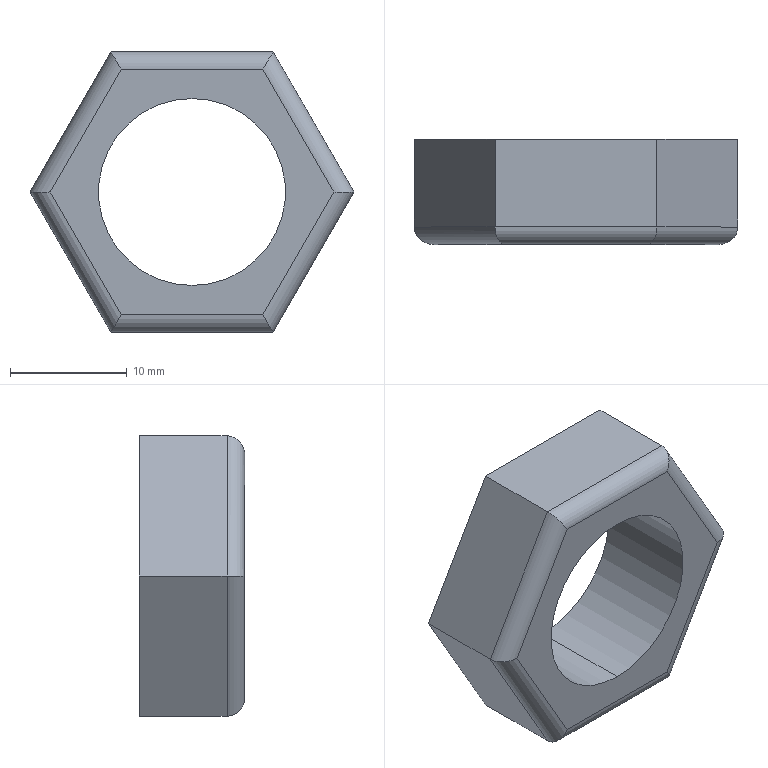Part | SolidWorks | features Extrusion 1, Fillet 1 | 1 solid | 16 faces | box 27.713 x 9 x 24 mm | volume 2641 mm3 | cylinder 8 | plane 8 | commonest cylinder face diameters 3 x6 16 x2
STEP:
#1=CARTESIAN_POINT('',(0.,9.,-8.));
#2=VERTEX_POINT('',#1);
#3=CARTESIAN_POINT('',(0.,9.,8.));
#4=VERTEX_POINT('',#3);
#5=CARTESIAN_POINT('',(0.,9.,0.));
#6=DIRECTION('',(0.,1.,0.));
#7=DIRECTION('',(0.,0.,1.));
#8=AXIS2_PLACEMENT_3D('',#5,#6,#7);
#9=CIRCLE('',#8,8.);
#10=EDGE_CURVE('',#2,#4,#9,.T.);
#11=ORIENTED_EDGE('',*,*,#10,.T.);
#12=CARTESIAN_POINT('',(0.,0.,8.));
#13=VERTEX_POINT('',#12);
#14=CARTESIAN_POINT('',(0.,9.,8.));
#15=DIRECTION('',(0.,-1.,0.));
#16=VECTOR('',#15,1000.);
#17=LINE('',#14,#16);
#18=EDGE_CURVE('',#4,#13,#17,.T.);
#19=ORIENTED_EDGE('',*,*,#18,.T.);
#20=CARTESIAN_POINT('',(0.,0.,-8.));
#21=VERTEX_POINT('',#20);
#22=CARTESIAN_POINT('',(0.,0.,0.));
#23=DIRECTION('',(0.,1.,0.));
#24=DIRECTION('',(0.,0.,1.));
#25=AXIS2_PLACEMENT_3D('',#22,#23,#24);
#26=CIRCLE('',#25,8.);
#27=EDGE_CURVE('',#21,#13,#26,.T.);
#28=ORIENTED_EDGE('',*,*,#27,.F.);
#29=CARTESIAN_POINT('',(0.,9.,-8.));
#30=DIRECTION('',(0.,-1.,0.));
#31=VECTOR('',#30,1000.);
#32=LINE('',#29,#31);
#33=EDGE_CURVE('',#2,#21,#32,.T.);
#34=ORIENTED_EDGE('',*,*,#33,.F.);
#35=EDGE_LOOP('',(#11,#19,#28,#34));
#36=FACE_OUTER_BOUND('',#35,.T.);
#37=CARTESIAN_POINT('',(0.,9.,0.));
#38=DIRECTION('',(0.,-1.,0.));
#39=DIRECTION('',(0.,0.,-1.));
#40=AXIS2_PLACEMENT_3D('',#37,#38,#39);
#41=CYLINDRICAL_SURFACE('',#40,8.);
#42=ADVANCED_FACE('',(#36),#41,.F.);
#43=CARTESIAN_POINT('',(6.928,9.,12.));
#44=VERTEX_POINT('',#43);
#45=CARTESIAN_POINT('',(13.856,9.,0.));
#46=VERTEX_POINT('',#45);
#47=CARTESIAN_POINT('',(6.928,9.,12.));
#48=DIRECTION('',(0.5,0.,-0.866));
#49=VECTOR('',#48,1000.);
#50=LINE('',#47,#49);
#51=EDGE_CURVE('',#44,#46,#50,.T.);
#52=ORIENTED_EDGE('',*,*,#51,.T.);
#53=CARTESIAN_POINT('',(6.928,9.,-12.));
#54=VERTEX_POINT('',#53);
#55=CARTESIAN_POINT('',(13.856,9.,0.));
#56=DIRECTION('',(-0.5,0.,-0.866));
#57=VECTOR('',#56,1000.);
#58=LINE('',#55,#57);
#59=EDGE_CURVE('',#46,#54,#58,.T.);
#60=ORIENTED_EDGE('',*,*,#59,.T.);
#61=CARTESIAN_POINT('',(-6.928,9.,-12.));
#62=VERTEX_POINT('',#61);
#63=CARTESIAN_POINT('',(6.928,9.,-12.));
#64=DIRECTION('',(-1.,0.,0.));
#65=VECTOR('',#64,1000.);
#66=LINE('',#63,#65);
#67=EDGE_CURVE('',#54,#62,#66,.T.);
#68=ORIENTED_EDGE('',*,*,#67,.T.);
#69=CARTESIAN_POINT('',(-13.856,9.,0.));
#70=VERTEX_POINT('',#69);
#71=CARTESIAN_POINT('',(-6.928,9.,-12.));
#72=DIRECTION('',(-0.5,0.,0.866));
#73=VECTOR('',#72,1000.);
#74=LINE('',#71,#73);
#75=EDGE_CURVE('',#62,#70,#74,.T.);
#76=ORIENTED_EDGE('',*,*,#75,.T.);
#77=CARTESIAN_POINT('',(-6.928,9.,12.));
#78=VERTEX_POINT('',#77);
#79=CARTESIAN_POINT('',(-13.856,9.,0.));
#80=DIRECTION('',(0.5,0.,0.866));
#81=VECTOR('',#80,1000.);
#82=LINE('',#79,#81);
#83=EDGE_CURVE('',#70,#78,#82,.T.);
#84=ORIENTED_EDGE('',*,*,#83,.T.);
#85=CARTESIAN_POINT('',(-6.928,9.,12.));
#86=DIRECTION('',(1.,0.,0.));
#87=VECTOR('',#86,1000.);
#88=LINE('',#85,#87);
#89=EDGE_CURVE('',#78,#44,#88,.T.);
#90=ORIENTED_EDGE('',*,*,#89,.T.);
#91=EDGE_LOOP('',(#52,#60,#68,#76,#84,#90));
#92=FACE_OUTER_BOUND('',#91,.T.);
#93=ORIENTED_EDGE('',*,*,#10,.F.);
#94=CARTESIAN_POINT('',(0.,9.,0.));
#95=DIRECTION('',(0.,1.,0.));
#96=DIRECTION('',(0.,0.,1.));
#97=AXIS2_PLACEMENT_3D('',#94,#95,#96);
#98=CIRCLE('',#97,8.);
#99=EDGE_CURVE('',#4,#2,#98,.T.);
#100=ORIENTED_EDGE('',*,*,#99,.F.);
#101=EDGE_LOOP('',(#93,#100));
#102=FACE_BOUND('',#101,.T.);
#103=CARTESIAN_POINT('',(13.856,9.,0.));
#104=DIRECTION('',(0.,1.,0.));
#105=DIRECTION('',(0.,0.,1.));
#106=AXIS2_PLACEMENT_3D('',#103,#104,#105);
#107=PLANE('',#106);
#108=ADVANCED_FACE('',(#92,#102),#107,.T.);
#109=CARTESIAN_POINT('',(-6.062,0.,-10.5));
#110=VERTEX_POINT('',#109);
#111=CARTESIAN_POINT('',(6.062,0.,-10.5));
#112=VERTEX_POINT('',#111);
#113=CARTESIAN_POINT('',(13.856,0.,-10.5));
#114=DIRECTION('',(1.,0.,0.));
#115=VECTOR('',#114,1000.);
#116=LINE('',#113,#115);
#117=EDGE_CURVE('',#110,#112,#116,.T.);
#118=ORIENTED_EDGE('',*,*,#117,.T.);
#119=CARTESIAN_POINT('',(12.124,0.,0.));
#120=VERTEX_POINT('',#119);
#121=CARTESIAN_POINT('',(12.557,0.,0.75));
#122=DIRECTION('',(0.5,0.,0.866));
#123=VECTOR('',#122,1000.);
#124=LINE('',#121,#123);
#125=EDGE_CURVE('',#112,#120,#124,.T.);
#126=ORIENTED_EDGE('',*,*,#125,.T.);
#127=CARTESIAN_POINT('',(6.062,0.,10.5));
#128=VERTEX_POINT('',#127);
#129=CARTESIAN_POINT('',(12.557,0.,-0.75));
#130=DIRECTION('',(-0.5,0.,0.866));
#131=VECTOR('',#130,1000.);
#132=LINE('',#129,#131);
#133=EDGE_CURVE('',#120,#128,#132,.T.);
#134=ORIENTED_EDGE('',*,*,#133,.T.);
#135=CARTESIAN_POINT('',(-6.062,0.,10.5));
#136=VERTEX_POINT('',#135);
#137=CARTESIAN_POINT('',(13.856,0.,10.5));
#138=DIRECTION('',(-1.,0.,0.));
#139=VECTOR('',#138,1000.);
#140=LINE('',#137,#139);
#141=EDGE_CURVE('',#128,#136,#140,.T.);
#142=ORIENTED_EDGE('',*,*,#141,.T.);
#143=CARTESIAN_POINT('',(-12.124,0.,0.));
#144=VERTEX_POINT('',#143);
#145=CARTESIAN_POINT('',(-5.629,0.,11.25));
#146=DIRECTION('',(-0.5,0.,-0.866));
#147=VECTOR('',#146,1000.);
#148=LINE('',#145,#147);
#149=EDGE_CURVE('',#136,#144,#148,.T.);
#150=ORIENTED_EDGE('',*,*,#149,.T.);
#151=CARTESIAN_POINT('',(-5.629,0.,-11.25));
#152=DIRECTION('',(0.5,0.,-0.866));
#153=VECTOR('',#152,1000.);
#154=LINE('',#151,#153);
#155=EDGE_CURVE('',#144,#110,#154,.T.);
#156=ORIENTED_EDGE('',*,*,#155,.T.);
#157=EDGE_LOOP('',(#118,#126,#134,#142,#150,#156));
#158=FACE_OUTER_BOUND('',#157,.T.);
#159=ORIENTED_EDGE('',*,*,#27,.T.);
#160=CARTESIAN_POINT('',(0.,0.,0.));
#161=DIRECTION('',(0.,1.,0.));
#162=DIRECTION('',(0.,0.,1.));
#163=AXIS2_PLACEMENT_3D('',#160,#161,#162);
#164=CIRCLE('',#163,8.);
#165=EDGE_CURVE('',#13,#21,#164,.T.);
#166=ORIENTED_EDGE('',*,*,#165,.T.);
#167=EDGE_LOOP('',(#159,#166));
#168=FACE_BOUND('',#167,.T.);
#169=CARTESIAN_POINT('',(13.856,0.,0.));
#170=DIRECTION('',(0.,1.,0.));
#171=DIRECTION('',(0.,0.,1.));
#172=AXIS2_PLACEMENT_3D('',#169,#170,#171);
#173=PLANE('',#172);
#174=ADVANCED_FACE('',(#158,#168),#173,.F.);
#175=CARTESIAN_POINT('',(6.928,1.5,12.));
#176=VERTEX_POINT('',#175);
#177=CARTESIAN_POINT('',(6.928,9.,12.));
#178=DIRECTION('',(0.,-1.,0.));
#179=VECTOR('',#178,1000.);
#180=LINE('',#177,#179);
#181=EDGE_CURVE('',#44,#176,#180,.T.);
#182=ORIENTED_EDGE('',*,*,#181,.T.);
#183=CARTESIAN_POINT('',(13.856,1.5,0.));
#184=VERTEX_POINT('',#183);
#185=CARTESIAN_POINT('',(6.928,1.5,12.));
#186=DIRECTION('',(0.5,0.,-0.866));
#187=VECTOR('',#186,1000.);
#188=LINE('',#185,#187);
#189=EDGE_CURVE('',#176,#184,#188,.T.);
#190=ORIENTED_EDGE('',*,*,#189,.T.);
#191=CARTESIAN_POINT('',(13.856,9.,0.));
#192=DIRECTION('',(0.,-1.,0.));
#193=VECTOR('',#192,1000.);
#194=LINE('',#191,#193);
#195=EDGE_CURVE('',#46,#184,#194,.T.);
#196=ORIENTED_EDGE('',*,*,#195,.F.);
#197=ORIENTED_EDGE('',*,*,#51,.F.);
#198=EDGE_LOOP('',(#182,#190,#196,#197));
#199=FACE_OUTER_BOUND('',#198,.T.);
#200=CARTESIAN_POINT('',(6.928,9.,12.));
#201=DIRECTION('',(-0.866,0.,-0.5));
#202=DIRECTION('',(-0.5,0.,0.866));
#203=AXIS2_PLACEMENT_3D('',#200,#201,#202);
#204=PLANE('',#203);
#205=ADVANCED_FACE('',(#199),#204,.F.);
#206=ORIENTED_EDGE('',*,*,#195,.T.);
#207=CARTESIAN_POINT('',(6.928,1.5,-12.));
#208=VERTEX_POINT('',#207);
#209=CARTESIAN_POINT('',(13.856,1.5,0.));
#210=DIRECTION('',(-0.5,0.,-0.866));
#211=VECTOR('',#210,1000.);
#212=LINE('',#209,#211);
#213=EDGE_CURVE('',#184,#208,#212,.T.);
#214=ORIENTED_EDGE('',*,*,#213,.T.);
#215=CARTESIAN_POINT('',(6.928,9.,-12.));
#216=DIRECTION('',(0.,-1.,0.));
#217=VECTOR('',#216,1000.);
#218=LINE('',#215,#217);
#219=EDGE_CURVE('',#54,#208,#218,.T.);
#220=ORIENTED_EDGE('',*,*,#219,.F.);
#221=ORIENTED_EDGE('',*,*,#59,.F.);
#222=EDGE_LOOP('',(#206,#214,#220,#221));
#223=FACE_OUTER_BOUND('',#222,.T.);
#224=CARTESIAN_POINT('',(13.856,9.,0.));
#225=DIRECTION('',(-0.866,0.,0.5));
#226=DIRECTION('',(0.5,0.,0.866));
#227=AXIS2_PLACEMENT_3D('',#224,#225,#226);
#228=PLANE('',#227);
#229=ADVANCED_FACE('',(#223),#228,.F.);
#230=ORIENTED_EDGE('',*,*,#219,.T.);
#231=CARTESIAN_POINT('',(-6.928,1.5,-12.));
#232=VERTEX_POINT('',#231);
#233=CARTESIAN_POINT('',(6.928,1.5,-12.));
#234=DIRECTION('',(-1.,0.,0.));
#235=VECTOR('',#234,1000.);
#236=LINE('',#233,#235);
#237=EDGE_CURVE('',#208,#232,#236,.T.);
#238=ORIENTED_EDGE('',*,*,#237,.T.);
#239=CARTESIAN_POINT('',(-6.928,9.,-12.));
#240=DIRECTION('',(0.,-1.,0.));
#241=VECTOR('',#240,1000.);
#242=LINE('',#239,#241);
#243=EDGE_CURVE('',#62,#232,#242,.T.);
#244=ORIENTED_EDGE('',*,*,#243,.F.);
#245=ORIENTED_EDGE('',*,*,#67,.F.);
#246=EDGE_LOOP('',(#230,#238,#244,#245));
#247=FACE_OUTER_BOUND('',#246,.T.);
#248=CARTESIAN_POINT('',(6.928,9.,-12.));
#249=DIRECTION('',(0.,0.,1.));
#250=DIRECTION('',(1.,0.,0.));
#251=AXIS2_PLACEMENT_3D('',#248,#249,#250);
#252=PLANE('',#251);
#253=ADVANCED_FACE('',(#247),#252,.F.);
#254=ORIENTED_EDGE('',*,*,#243,.T.);
#255=CARTESIAN_POINT('',(-13.856,1.5,0.));
#256=VERTEX_POINT('',#255);
#257=CARTESIAN_POINT('',(-6.928,1.5,-12.));
#258=DIRECTION('',(-0.5,0.,0.866));
#259=VECTOR('',#258,1000.);
#260=LINE('',#257,#259);
#261=EDGE_CURVE('',#232,#256,#260,.T.);
#262=ORIENTED_EDGE('',*,*,#261,.T.);
#263=CARTESIAN_POINT('',(-13.856,9.,0.));
#264=DIRECTION('',(0.,-1.,0.));
#265=VECTOR('',#264,1000.);
#266=LINE('',#263,#265);
#267=EDGE_CURVE('',#70,#256,#266,.T.);
#268=ORIENTED_EDGE('',*,*,#267,.F.);
#269=ORIENTED_EDGE('',*,*,#75,.F.);
#270=EDGE_LOOP('',(#254,#262,#268,#269));
#271=FACE_OUTER_BOUND('',#270,.T.);
#272=CARTESIAN_POINT('',(-6.928,9.,-12.));
#273=DIRECTION('',(0.866,0.,0.5));
#274=DIRECTION('',(0.5,0.,-0.866));
#275=AXIS2_PLACEMENT_3D('',#272,#273,#274);
#276=PLANE('',#275);
#277=ADVANCED_FACE('',(#271),#276,.F.);
#278=ORIENTED_EDGE('',*,*,#267,.T.);
#279=CARTESIAN_POINT('',(-6.928,1.5,12.));
#280=VERTEX_POINT('',#279);
#281=CARTESIAN_POINT('',(-13.856,1.5,0.));
#282=DIRECTION('',(0.5,0.,0.866));
#283=VECTOR('',#282,1000.);
#284=LINE('',#281,#283);
#285=EDGE_CURVE('',#256,#280,#284,.T.);
#286=ORIENTED_EDGE('',*,*,#285,.T.);
#287=CARTESIAN_POINT('',(-6.928,9.,12.));
#288=DIRECTION('',(0.,-1.,0.));
#289=VECTOR('',#288,1000.);
#290=LINE('',#287,#289);
#291=EDGE_CURVE('',#78,#280,#290,.T.);
#292=ORIENTED_EDGE('',*,*,#291,.F.);
#293=ORIENTED_EDGE('',*,*,#83,.F.);
#294=EDGE_LOOP('',(#278,#286,#292,#293));
#295=FACE_OUTER_BOUND('',#294,.T.);
#296=CARTESIAN_POINT('',(-13.856,9.,0.));
#297=DIRECTION('',(0.866,0.,-0.5));
#298=DIRECTION('',(-0.5,0.,-0.866));
#299=AXIS2_PLACEMENT_3D('',#296,#297,#298);
#300=PLANE('',#299);
#301=ADVANCED_FACE('',(#295),#300,.F.);
#302=ORIENTED_EDGE('',*,*,#291,.T.);
#303=CARTESIAN_POINT('',(-6.928,1.5,12.));
#304=DIRECTION('',(1.,0.,0.));
#305=VECTOR('',#304,1000.);
#306=LINE('',#303,#305);
#307=EDGE_CURVE('',#280,#176,#306,.T.);
#308=ORIENTED_EDGE('',*,*,#307,.T.);
#309=ORIENTED_EDGE('',*,*,#181,.F.);
#310=ORIENTED_EDGE('',*,*,#89,.F.);
#311=EDGE_LOOP('',(#302,#308,#309,#310));
#312=FACE_OUTER_BOUND('',#311,.T.);
#313=CARTESIAN_POINT('',(-6.928,9.,12.));
#314=DIRECTION('',(0.,0.,-1.));
#315=DIRECTION('',(-1.,0.,0.));
#316=AXIS2_PLACEMENT_3D('',#313,#314,#315);
#317=PLANE('',#316);
#318=ADVANCED_FACE('',(#312),#317,.F.);
#319=ORIENTED_EDGE('',*,*,#18,.F.);
#320=ORIENTED_EDGE('',*,*,#99,.T.);
#321=ORIENTED_EDGE('',*,*,#33,.T.);
#322=ORIENTED_EDGE('',*,*,#165,.F.);
#323=EDGE_LOOP('',(#319,#320,#321,#322));
#324=FACE_OUTER_BOUND('',#323,.T.);
#325=CARTESIAN_POINT('',(0.,9.,0.));
#326=DIRECTION('',(0.,-1.,0.));
#327=DIRECTION('',(0.,0.,-1.));
#328=AXIS2_PLACEMENT_3D('',#325,#326,#327);
#329=CYLINDRICAL_SURFACE('',#328,8.);
#330=ADVANCED_FACE('',(#324),#329,.F.);
#331=CARTESIAN_POINT('',(-12.124,0.,0.));
#332=CARTESIAN_POINT('',(-13.139,0.,0.));
#333=CARTESIAN_POINT('',(-13.856,0.6213,0.));
#334=CARTESIAN_POINT('',(-13.856,1.5,0.));
#335=(BOUNDED_CURVE()B_SPLINE_CURVE(3,(#331,#332,#333,#334),.UNSPECIFIED.,.F.,.T.)B_SPLINE_CURVE_WITH_KNOTS((4,4),(4.712,6.283),.UNSPECIFIED.)CURVE()GEOMETRIC_REPRESENTATION_ITEM()RATIONAL_B_SPLINE_CURVE((1.,0.8047,0.8047,1.))REPRESENTATION_ITEM(''));
#336=EDGE_CURVE('',#144,#256,#335,.T.);
#337=ORIENTED_EDGE('',*,*,#336,.F.);
#338=ORIENTED_EDGE('',*,*,#149,.F.);
#339=CARTESIAN_POINT('',(-6.928,1.5,12.));
#340=CARTESIAN_POINT('',(-6.928,0.6213,12.));
#341=CARTESIAN_POINT('',(-6.569,0.,11.379));
#342=CARTESIAN_POINT('',(-6.062,0.,10.5));
#343=(BOUNDED_CURVE()B_SPLINE_CURVE(3,(#339,#340,#341,#342),.UNSPECIFIED.,.F.,.F.)B_SPLINE_CURVE_WITH_KNOTS((4,4),(0.,1.571),.UNSPECIFIED.)CURVE()GEOMETRIC_REPRESENTATION_ITEM()RATIONAL_B_SPLINE_CURVE((1.,0.8047,0.8047,1.))REPRESENTATION_ITEM(''));
#344=EDGE_CURVE('',#280,#136,#343,.T.);
#345=ORIENTED_EDGE('',*,*,#344,.F.);
#346=ORIENTED_EDGE('',*,*,#285,.F.);
#347=EDGE_LOOP('',(#337,#338,#345,#346));
#348=FACE_OUTER_BOUND('',#347,.T.);
#349=CARTESIAN_POINT('',(-12.557,1.5,-0.75));
#350=DIRECTION('',(0.5,0.,0.866));
#351=DIRECTION('',(0.866,0.,-0.5));
#352=AXIS2_PLACEMENT_3D('',#349,#350,#351);
#353=CYLINDRICAL_SURFACE('',#352,1.5);
#354=ADVANCED_FACE('',(#348),#353,.T.);
#355=ORIENTED_EDGE('',*,*,#344,.T.);
#356=ORIENTED_EDGE('',*,*,#141,.F.);
#357=CARTESIAN_POINT('',(6.928,1.5,12.));
#358=CARTESIAN_POINT('',(6.928,0.6213,12.));
#359=CARTESIAN_POINT('',(6.569,0.,11.379));
#360=CARTESIAN_POINT('',(6.062,0.,10.5));
#361=(BOUNDED_CURVE()B_SPLINE_CURVE(3,(#357,#358,#359,#360),.UNSPECIFIED.,.F.,.F.)B_SPLINE_CURVE_WITH_KNOTS((4,4),(0.,1.571),.UNSPECIFIED.)CURVE()GEOMETRIC_REPRESENTATION_ITEM()RATIONAL_B_SPLINE_CURVE((1.,0.8047,0.8047,1.))REPRESENTATION_ITEM(''));
#362=EDGE_CURVE('',#176,#128,#361,.T.);
#363=ORIENTED_EDGE('',*,*,#362,.F.);
#364=ORIENTED_EDGE('',*,*,#307,.F.);
#365=EDGE_LOOP('',(#355,#356,#363,#364));
#366=FACE_OUTER_BOUND('',#365,.T.);
#367=CARTESIAN_POINT('',(-6.928,1.5,10.5));
#368=DIRECTION('',(1.,0.,0.));
#369=DIRECTION('',(0.,0.,-1.));
#370=AXIS2_PLACEMENT_3D('',#367,#368,#369);
#371=CYLINDRICAL_SURFACE('',#370,1.5);
#372=ADVANCED_FACE('',(#366),#371,.T.);
#373=ORIENTED_EDGE('',*,*,#336,.T.);
#374=ORIENTED_EDGE('',*,*,#261,.F.);
#375=CARTESIAN_POINT('',(-6.062,0.,-10.5));
#376=CARTESIAN_POINT('',(-6.569,0.,-11.379));
#377=CARTESIAN_POINT('',(-6.928,0.6213,-12.));
#378=CARTESIAN_POINT('',(-6.928,1.5,-12.));
#379=(BOUNDED_CURVE()B_SPLINE_CURVE(3,(#375,#376,#377,#378),.UNSPECIFIED.,.F.,.F.)B_SPLINE_CURVE_WITH_KNOTS((4,4),(4.712,6.283),.UNSPECIFIED.)CURVE()GEOMETRIC_REPRESENTATION_ITEM()RATIONAL_B_SPLINE_CURVE((1.,0.8047,0.8047,1.))REPRESENTATION_ITEM(''));
#380=EDGE_CURVE('',#110,#232,#379,.T.);
#381=ORIENTED_EDGE('',*,*,#380,.F.);
#382=ORIENTED_EDGE('',*,*,#155,.F.);
#383=EDGE_LOOP('',(#373,#374,#381,#382));
#384=FACE_OUTER_BOUND('',#383,.T.);
#385=CARTESIAN_POINT('',(-5.629,1.5,-11.25));
#386=DIRECTION('',(-0.5,0.,0.866));
#387=DIRECTION('',(0.866,0.,0.5));
#388=AXIS2_PLACEMENT_3D('',#385,#386,#387);
#389=CYLINDRICAL_SURFACE('',#388,1.5);
#390=ADVANCED_FACE('',(#384),#389,.T.);
#391=ORIENTED_EDGE('',*,*,#362,.T.);
#392=ORIENTED_EDGE('',*,*,#133,.F.);
#393=CARTESIAN_POINT('',(13.856,1.5,0.));
#394=CARTESIAN_POINT('',(13.856,0.6213,0.));
#395=CARTESIAN_POINT('',(13.139,0.,0.));
#396=CARTESIAN_POINT('',(12.124,0.,0.));
#397=(BOUNDED_CURVE()B_SPLINE_CURVE(3,(#393,#394,#395,#396),.UNSPECIFIED.,.F.,.T.)B_SPLINE_CURVE_WITH_KNOTS((4,4),(0.,1.571),.UNSPECIFIED.)CURVE()GEOMETRIC_REPRESENTATION_ITEM()RATIONAL_B_SPLINE_CURVE((1.,0.8047,0.8047,1.))REPRESENTATION_ITEM(''));
#398=EDGE_CURVE('',#184,#120,#397,.T.);
#399=ORIENTED_EDGE('',*,*,#398,.F.);
#400=ORIENTED_EDGE('',*,*,#189,.F.);
#401=EDGE_LOOP('',(#391,#392,#399,#400));
#402=FACE_OUTER_BOUND('',#401,.T.);
#403=CARTESIAN_POINT('',(5.629,1.5,11.25));
#404=DIRECTION('',(0.5,0.,-0.866));
#405=DIRECTION('',(-0.866,0.,-0.5));
#406=AXIS2_PLACEMENT_3D('',#403,#404,#405);
#407=CYLINDRICAL_SURFACE('',#406,1.5);
#408=ADVANCED_FACE('',(#402),#407,.T.);
#409=ORIENTED_EDGE('',*,*,#380,.T.);
#410=ORIENTED_EDGE('',*,*,#237,.F.);
#411=CARTESIAN_POINT('',(6.062,0.,-10.5));
#412=CARTESIAN_POINT('',(6.569,0.,-11.379));
#413=CARTESIAN_POINT('',(6.928,0.6213,-12.));
#414=CARTESIAN_POINT('',(6.928,1.5,-12.));
#415=(BOUNDED_CURVE()B_SPLINE_CURVE(3,(#411,#412,#413,#414),.UNSPECIFIED.,.F.,.F.)B_SPLINE_CURVE_WITH_KNOTS((4,4),(1.571,3.142),.UNSPECIFIED.)CURVE()GEOMETRIC_REPRESENTATION_ITEM()RATIONAL_B_SPLINE_CURVE((1.,0.8047,0.8047,1.))REPRESENTATION_ITEM(''));
#416=EDGE_CURVE('',#112,#208,#415,.T.);
#417=ORIENTED_EDGE('',*,*,#416,.F.);
#418=ORIENTED_EDGE('',*,*,#117,.F.);
#419=EDGE_LOOP('',(#409,#410,#417,#418));
#420=FACE_OUTER_BOUND('',#419,.T.);
#421=CARTESIAN_POINT('',(6.928,1.5,-10.5));
#422=DIRECTION('',(-1.,0.,0.));
#423=DIRECTION('',(0.,0.,1.));
#424=AXIS2_PLACEMENT_3D('',#421,#422,#423);
#425=CYLINDRICAL_SURFACE('',#424,1.5);
#426=ADVANCED_FACE('',(#420),#425,.T.);
#427=ORIENTED_EDGE('',*,*,#398,.T.);
#428=ORIENTED_EDGE('',*,*,#125,.F.);
#429=ORIENTED_EDGE('',*,*,#416,.T.);
#430=ORIENTED_EDGE('',*,*,#213,.F.);
#431=EDGE_LOOP('',(#427,#428,#429,#430));
#432=FACE_OUTER_BOUND('',#431,.T.);
#433=CARTESIAN_POINT('',(12.557,1.5,0.75));
#434=DIRECTION('',(-0.5,0.,-0.866));
#435=DIRECTION('',(-0.866,0.,0.5));
#436=AXIS2_PLACEMENT_3D('',#433,#434,#435);
#437=CYLINDRICAL_SURFACE('',#436,1.5);
#438=ADVANCED_FACE('',(#432),#437,.T.);
#439=CLOSED_SHELL('',(#42,#108,#174,#205,#229,#253,#277,#301,#318,#330,#354,#372,#390,#408,#426,#438));
#440=MANIFOLD_SOLID_BREP('',#439);
#441=CARTESIAN_POINT('',(0.,0.,0.));
#442=DIRECTION('',(0.,0.,1.));
#443=DIRECTION('',(1.,0.,0.));
#444=AXIS2_PLACEMENT_3D('',#441,#442,#443);
#445=(LENGTH_UNIT()NAMED_UNIT(*)SI_UNIT(.MILLI.,.METRE.));
#446=UNCERTAINTY_MEASURE_WITH_UNIT(LENGTH_MEASURE(0.00001),#445,'','');
#447=(NAMED_UNIT(*)PLANE_ANGLE_UNIT()SI_UNIT($,.RADIAN.));
#448=(NAMED_UNIT(*)SI_UNIT($,.STERADIAN.)SOLID_ANGLE_UNIT());
#449=(GEOMETRIC_REPRESENTATION_CONTEXT(3)GLOBAL_UNCERTAINTY_ASSIGNED_CONTEXT((#446))GLOBAL_UNIT_ASSIGNED_CONTEXT((#445,#447,#448))REPRESENTATION_CONTEXT('',''));
#450=ADVANCED_BREP_SHAPE_REPRESENTATION('',(#440,#444),#449);